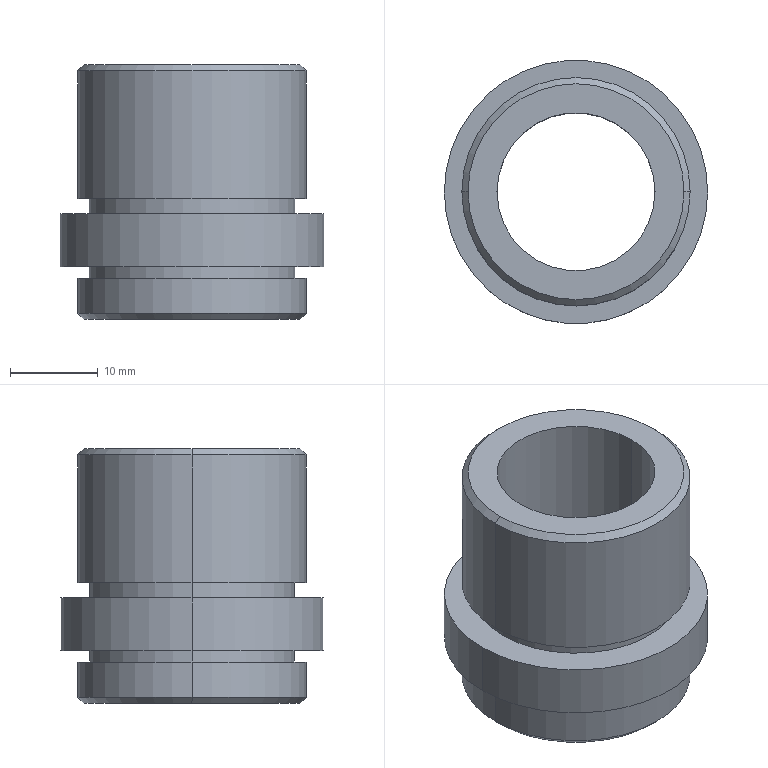Part | STEP file | TBW-1812 | 1 solid | 22 faces | box 30 x 30 x 29 mm | volume 8727 mm3 | cylinder 12 | plane 6 | cone 4 | commonest cylinder face diameters 23.4 x4 26 x4 18 x2 30 x2
STEP:
#1=CARTESIAN_POINT('',(0.,0.,0.));
#2=DIRECTION('',(0.,0.,1.));
#3=DIRECTION('',(1.,0.,0.));
#4=AXIS2_PLACEMENT_3D('',#1,#2,#3);
#5=CARTESIAN_POINT('',(-9.,0.,29.));
#6=VERTEX_POINT('',#5);
#7=CARTESIAN_POINT('',(-9.,0.,0.));
#8=VERTEX_POINT('',#7);
#9=CARTESIAN_POINT('',(-9.,0.,14.5));
#10=DIRECTION('',(0.,0.,-1.));
#11=VECTOR('',#10,1.);
#12=LINE('',#9,#11);
#13=CARTESIAN_POINT('',(0.,0.,14.5));
#14=DIRECTION('',(0.,0.,-1.));
#15=DIRECTION('',(-1.,0.,0.));
#16=AXIS2_PLACEMENT_3D('',#13,#14,#15);
#17=CYLINDRICAL_SURFACE('',#16,9.);
#18=CARTESIAN_POINT('',(6.283,0.));
#19=DIRECTION('',(0.,1.));
#20=VECTOR('',#19,1.);
#21=LINE('',#18,#20);
#22=(GEOMETRIC_REPRESENTATION_CONTEXT(2)PARAMETRIC_REPRESENTATION_CONTEXT()REPRESENTATION_CONTEXT('',''));
#23=DEFINITIONAL_REPRESENTATION('',(#21),#22);
#24=PCURVE('',#17,#23);
#25=CARTESIAN_POINT('',(0.,0.,14.5));
#26=DIRECTION('',(0.,0.,-1.));
#27=DIRECTION('',(-1.,0.,0.));
#28=AXIS2_PLACEMENT_3D('',#25,#26,#27);
#29=CYLINDRICAL_SURFACE('',#28,9.);
#30=CARTESIAN_POINT('',(0.,0.));
#31=DIRECTION('',(0.,1.));
#32=VECTOR('',#31,1.);
#33=LINE('',#30,#32);
#34=(GEOMETRIC_REPRESENTATION_CONTEXT(2)PARAMETRIC_REPRESENTATION_CONTEXT()REPRESENTATION_CONTEXT('',''));
#35=DEFINITIONAL_REPRESENTATION('',(#33),#34);
#36=PCURVE('',#29,#35);
#37=SURFACE_CURVE('',#12,(#24,#36),.PCURVE_S1.);
#38=EDGE_CURVE('',#6,#8,#37,.T.);
#39=ORIENTED_EDGE('',*,*,#38,.T.);
#40=CARTESIAN_POINT('',(9.,0.,0.));
#41=VERTEX_POINT('',#40);
#42=CARTESIAN_POINT('',(0.,0.,0.));
#43=DIRECTION('',(0.,0.,1.));
#44=DIRECTION('',(-1.,0.,0.));
#45=AXIS2_PLACEMENT_3D('',#42,#43,#44);
#46=CIRCLE('',#45,9.);
#47=CARTESIAN_POINT('',(6.283,14.5));
#48=DIRECTION('',(-1.,0.));
#49=VECTOR('',#48,1.);
#50=LINE('',#47,#49);
#51=(GEOMETRIC_REPRESENTATION_CONTEXT(2)PARAMETRIC_REPRESENTATION_CONTEXT()REPRESENTATION_CONTEXT('',''));
#52=DEFINITIONAL_REPRESENTATION('',(#50),#51);
#53=PCURVE('',#17,#52);
#54=CARTESIAN_POINT('',(0.,6.5,0.));
#55=DIRECTION('',(0.,0.,-1.));
#56=DIRECTION('',(-1.,0.,0.));
#57=AXIS2_PLACEMENT_3D('',#54,#55,#56);
#58=PLANE('',#57);
#59=CARTESIAN_POINT('',(9.,-6.5));
#60=CARTESIAN_POINT('',(9.,-22.088));
#61=CARTESIAN_POINT('',(-4.5,-14.294));
#62=CARTESIAN_POINT('',(-18.,-6.5));
#63=CARTESIAN_POINT('',(-4.5,1.294));
#64=CARTESIAN_POINT('',(9.,9.088));
#65=CARTESIAN_POINT('',(9.,-6.5));
#66=(BOUNDED_CURVE()B_SPLINE_CURVE(2,(#59,#60,#61,#62,#63,#64,#65),.UNSPECIFIED.,.T.,.F.)B_SPLINE_CURVE_WITH_KNOTS((1,2,2,2,2,1),(-2.094,0.,2.094,4.189,6.283,8.378),.UNSPECIFIED.)CURVE()GEOMETRIC_REPRESENTATION_ITEM()RATIONAL_B_SPLINE_CURVE((1.,0.5,1.,0.5,1.,0.5,1.))REPRESENTATION_ITEM(''));
#67=(GEOMETRIC_REPRESENTATION_CONTEXT(2)PARAMETRIC_REPRESENTATION_CONTEXT()REPRESENTATION_CONTEXT('',''));
#68=DEFINITIONAL_REPRESENTATION('',(#66),#67);
#69=PCURVE('',#58,#68);
#70=SURFACE_CURVE('',#46,(#53,#69),.PCURVE_S1.);
#71=EDGE_CURVE('',#8,#41,#70,.T.);
#72=ORIENTED_EDGE('',*,*,#71,.T.);
#73=CARTESIAN_POINT('',(9.,0.,29.));
#74=VERTEX_POINT('',#73);
#75=CARTESIAN_POINT('',(9.,0.,14.5));
#76=DIRECTION('',(0.,0.,-1.));
#77=VECTOR('',#76,1.);
#78=LINE('',#75,#77);
#79=CARTESIAN_POINT('',(3.142,0.));
#80=DIRECTION('',(0.,1.));
#81=VECTOR('',#80,1.);
#82=LINE('',#79,#81);
#83=(GEOMETRIC_REPRESENTATION_CONTEXT(2)PARAMETRIC_REPRESENTATION_CONTEXT()REPRESENTATION_CONTEXT('',''));
#84=DEFINITIONAL_REPRESENTATION('',(#82),#83);
#85=PCURVE('',#17,#84);
#86=CARTESIAN_POINT('',(3.142,0.));
#87=DIRECTION('',(0.,1.));
#88=VECTOR('',#87,1.);
#89=LINE('',#86,#88);
#90=(GEOMETRIC_REPRESENTATION_CONTEXT(2)PARAMETRIC_REPRESENTATION_CONTEXT()REPRESENTATION_CONTEXT('',''));
#91=DEFINITIONAL_REPRESENTATION('',(#89),#90);
#92=PCURVE('',#29,#91);
#93=SURFACE_CURVE('',#78,(#85,#92),.PCURVE_S1.);
#94=EDGE_CURVE('',#74,#41,#93,.T.);
#95=ORIENTED_EDGE('',*,*,#94,.F.);
#96=CARTESIAN_POINT('',(0.,0.,29.));
#97=DIRECTION('',(0.,0.,-1.));
#98=DIRECTION('',(-1.,0.,0.));
#99=AXIS2_PLACEMENT_3D('',#96,#97,#98);
#100=CIRCLE('',#99,9.);
#101=CARTESIAN_POINT('',(0.,-14.5));
#102=DIRECTION('',(1.,0.));
#103=VECTOR('',#102,1.);
#104=LINE('',#101,#103);
#105=(GEOMETRIC_REPRESENTATION_CONTEXT(2)PARAMETRIC_REPRESENTATION_CONTEXT()REPRESENTATION_CONTEXT('',''));
#106=DEFINITIONAL_REPRESENTATION('',(#104),#105);
#107=PCURVE('',#17,#106);
#108=CARTESIAN_POINT('',(0.,6.5,29.));
#109=DIRECTION('',(0.,0.,1.));
#110=DIRECTION('',(1.,0.,0.));
#111=AXIS2_PLACEMENT_3D('',#108,#109,#110);
#112=PLANE('',#111);
#113=CARTESIAN_POINT('',(-9.,-6.5));
#114=CARTESIAN_POINT('',(-9.,9.088));
#115=CARTESIAN_POINT('',(4.5,1.294));
#116=CARTESIAN_POINT('',(18.,-6.5));
#117=CARTESIAN_POINT('',(4.5,-14.294));
#118=CARTESIAN_POINT('',(-9.,-22.088));
#119=CARTESIAN_POINT('',(-9.,-6.5));
#120=(BOUNDED_CURVE()B_SPLINE_CURVE(2,(#113,#114,#115,#116,#117,#118,#119),.UNSPECIFIED.,.T.,.F.)B_SPLINE_CURVE_WITH_KNOTS((1,2,2,2,2,1),(-2.094,0.,2.094,4.189,6.283,8.378),.UNSPECIFIED.)CURVE()GEOMETRIC_REPRESENTATION_ITEM()RATIONAL_B_SPLINE_CURVE((1.,0.5,1.,0.5,1.,0.5,1.))REPRESENTATION_ITEM(''));
#121=(GEOMETRIC_REPRESENTATION_CONTEXT(2)PARAMETRIC_REPRESENTATION_CONTEXT()REPRESENTATION_CONTEXT('',''));
#122=DEFINITIONAL_REPRESENTATION('',(#120),#121);
#123=PCURVE('',#112,#122);
#124=SURFACE_CURVE('',#100,(#107,#123),.PCURVE_S1.);
#125=EDGE_CURVE('',#74,#6,#124,.T.);
#126=ORIENTED_EDGE('',*,*,#125,.T.);
#127=EDGE_LOOP('',(#39,#72,#95,#126));
#128=FACE_BOUND('',#127,.F.);
#129=ADVANCED_FACE('',(#128),#17,.F.);
#130=CARTESIAN_POINT('',(12.293,0.,29.));
#131=VERTEX_POINT('',#130);
#132=CARTESIAN_POINT('',(-12.293,0.,29.));
#133=VERTEX_POINT('',#132);
#134=CARTESIAN_POINT('',(0.,0.,29.));
#135=DIRECTION('',(0.,0.,1.));
#136=DIRECTION('',(-1.,0.,0.));
#137=AXIS2_PLACEMENT_3D('',#134,#135,#136);
#138=CIRCLE('',#137,12.293);
#139=CARTESIAN_POINT('',(0.,0.,28.293));
#140=DIRECTION('',(0.,0.,-1.));
#141=DIRECTION('',(-1.,0.,0.));
#142=AXIS2_PLACEMENT_3D('',#139,#140,#141);
#143=CONICAL_SURFACE('',#142,13.,0.7854);
#144=CARTESIAN_POINT('',(6.283,-0.7071));
#145=DIRECTION('',(-1.,0.));
#146=VECTOR('',#145,1.);
#147=LINE('',#144,#146);
#148=(GEOMETRIC_REPRESENTATION_CONTEXT(2)PARAMETRIC_REPRESENTATION_CONTEXT()REPRESENTATION_CONTEXT('',''));
#149=DEFINITIONAL_REPRESENTATION('',(#147),#148);
#150=PCURVE('',#143,#149);
#151=CARTESIAN_POINT('',(0.,-6.5));
#152=DIRECTION('',(-1.,0.));
#153=AXIS2_PLACEMENT_2D('',#151,#152);
#154=CIRCLE('',#153,12.293);
#155=(GEOMETRIC_REPRESENTATION_CONTEXT(2)PARAMETRIC_REPRESENTATION_CONTEXT()REPRESENTATION_CONTEXT('',''));
#156=DEFINITIONAL_REPRESENTATION('',(#154),#155);
#157=PCURVE('',#112,#156);
#158=SURFACE_CURVE('',#138,(#150,#157),.PCURVE_S1.);
#159=EDGE_CURVE('',#131,#133,#158,.T.);
#160=ORIENTED_EDGE('',*,*,#159,.F.);
#161=CARTESIAN_POINT('',(13.,0.,28.293));
#162=VERTEX_POINT('',#161);
#163=CARTESIAN_POINT('',(13.,0.,28.293));
#164=DIRECTION('',(0.7071,0.,-0.7071));
#165=VECTOR('',#164,1.);
#166=LINE('',#163,#165);
#167=CARTESIAN_POINT('',(3.142,0.));
#168=DIRECTION('',(0.,1.));
#169=VECTOR('',#168,1.);
#170=LINE('',#167,#169);
#171=(GEOMETRIC_REPRESENTATION_CONTEXT(2)PARAMETRIC_REPRESENTATION_CONTEXT()REPRESENTATION_CONTEXT('',''));
#172=DEFINITIONAL_REPRESENTATION('',(#170),#171);
#173=PCURVE('',#143,#172);
#174=CARTESIAN_POINT('',(0.,0.,28.293));
#175=DIRECTION('',(0.,0.,-1.));
#176=DIRECTION('',(-1.,0.,0.));
#177=AXIS2_PLACEMENT_3D('',#174,#175,#176);
#178=CONICAL_SURFACE('',#177,13.,0.7854);
#179=CARTESIAN_POINT('',(3.142,0.));
#180=DIRECTION('',(0.,1.));
#181=VECTOR('',#180,1.);
#182=LINE('',#179,#181);
#183=(GEOMETRIC_REPRESENTATION_CONTEXT(2)PARAMETRIC_REPRESENTATION_CONTEXT()REPRESENTATION_CONTEXT('',''));
#184=DEFINITIONAL_REPRESENTATION('',(#182),#183);
#185=PCURVE('',#178,#184);
#186=SURFACE_CURVE('',#166,(#173,#185),.PCURVE_S1.);
#187=EDGE_CURVE('',#131,#162,#186,.T.);
#188=ORIENTED_EDGE('',*,*,#187,.T.);
#189=CARTESIAN_POINT('',(-13.,0.,28.293));
#190=VERTEX_POINT('',#189);
#191=CARTESIAN_POINT('',(0.,0.,28.293));
#192=DIRECTION('',(0.,0.,1.));
#193=DIRECTION('',(0.,1.,0.));
#194=AXIS2_PLACEMENT_3D('',#191,#192,#193);
#195=CIRCLE('',#194,13.);
#196=CARTESIAN_POINT('',(7.854,0.));
#197=DIRECTION('',(-1.,0.));
#198=VECTOR('',#197,1.);
#199=LINE('',#196,#198);
#200=(GEOMETRIC_REPRESENTATION_CONTEXT(2)PARAMETRIC_REPRESENTATION_CONTEXT()REPRESENTATION_CONTEXT('',''));
#201=DEFINITIONAL_REPRESENTATION('',(#199),#200);
#202=PCURVE('',#143,#201);
#203=CARTESIAN_POINT('',(0.,0.,20.5));
#204=DIRECTION('',(0.,0.,-1.));
#205=DIRECTION('',(-1.,0.,0.));
#206=AXIS2_PLACEMENT_3D('',#203,#204,#205);
#207=CYLINDRICAL_SURFACE('',#206,13.);
#208=CARTESIAN_POINT('',(7.854,-7.793));
#209=DIRECTION('',(-1.,0.));
#210=VECTOR('',#209,1.);
#211=LINE('',#208,#210);
#212=(GEOMETRIC_REPRESENTATION_CONTEXT(2)PARAMETRIC_REPRESENTATION_CONTEXT()REPRESENTATION_CONTEXT('',''));
#213=DEFINITIONAL_REPRESENTATION('',(#211),#212);
#214=PCURVE('',#207,#213);
#215=SURFACE_CURVE('',#195,(#202,#214),.PCURVE_S1.);
#216=EDGE_CURVE('',#162,#190,#215,.T.);
#217=ORIENTED_EDGE('',*,*,#216,.T.);
#218=CARTESIAN_POINT('',(-13.,0.,28.293));
#219=DIRECTION('',(-0.7071,0.,-0.7071));
#220=VECTOR('',#219,1.);
#221=LINE('',#218,#220);
#222=CARTESIAN_POINT('',(0.,0.));
#223=DIRECTION('',(0.,1.));
#224=VECTOR('',#223,1.);
#225=LINE('',#222,#224);
#226=(GEOMETRIC_REPRESENTATION_CONTEXT(2)PARAMETRIC_REPRESENTATION_CONTEXT()REPRESENTATION_CONTEXT('',''));
#227=DEFINITIONAL_REPRESENTATION('',(#225),#226);
#228=PCURVE('',#143,#227);
#229=CARTESIAN_POINT('',(6.283,0.));
#230=DIRECTION('',(0.,1.));
#231=VECTOR('',#230,1.);
#232=LINE('',#229,#231);
#233=(GEOMETRIC_REPRESENTATION_CONTEXT(2)PARAMETRIC_REPRESENTATION_CONTEXT()REPRESENTATION_CONTEXT('',''));
#234=DEFINITIONAL_REPRESENTATION('',(#232),#233);
#235=PCURVE('',#178,#234);
#236=SURFACE_CURVE('',#221,(#228,#235),.PCURVE_S1.);
#237=EDGE_CURVE('',#133,#190,#236,.T.);
#238=ORIENTED_EDGE('',*,*,#237,.F.);
#239=EDGE_LOOP('',(#160,#188,#217,#238));
#240=FACE_BOUND('',#239,.T.);
#241=ADVANCED_FACE('',(#240),#143,.T.);
#242=CARTESIAN_POINT('',(-12.293,0.,0.));
#243=VERTEX_POINT('',#242);
#244=CARTESIAN_POINT('',(12.293,0.,0.));
#245=VERTEX_POINT('',#244);
#246=CARTESIAN_POINT('',(0.,0.,0.));
#247=DIRECTION('',(0.,0.,-1.));
#248=DIRECTION('',(1.,0.,0.));
#249=AXIS2_PLACEMENT_3D('',#246,#247,#248);
#250=CIRCLE('',#249,12.293);
#251=CARTESIAN_POINT('',(0.,0.,0.7071));
#252=DIRECTION('',(0.,0.,1.));
#253=DIRECTION('',(1.,0.,0.));
#254=AXIS2_PLACEMENT_3D('',#251,#252,#253);
#255=CONICAL_SURFACE('',#254,13.,0.7854);
#256=CARTESIAN_POINT('',(6.283,-0.7071));
#257=DIRECTION('',(-1.,0.));
#258=VECTOR('',#257,1.);
#259=LINE('',#256,#258);
#260=(GEOMETRIC_REPRESENTATION_CONTEXT(2)PARAMETRIC_REPRESENTATION_CONTEXT()REPRESENTATION_CONTEXT('',''));
#261=DEFINITIONAL_REPRESENTATION('',(#259),#260);
#262=PCURVE('',#255,#261);
#263=CARTESIAN_POINT('',(0.,-6.5));
#264=DIRECTION('',(-1.,0.));
#265=AXIS2_PLACEMENT_2D('',#263,#264);
#266=CIRCLE('',#265,12.293);
#267=(GEOMETRIC_REPRESENTATION_CONTEXT(2)PARAMETRIC_REPRESENTATION_CONTEXT()REPRESENTATION_CONTEXT('',''));
#268=DEFINITIONAL_REPRESENTATION('',(#266),#267);
#269=PCURVE('',#58,#268);
#270=SURFACE_CURVE('',#250,(#262,#269),.PCURVE_S1.);
#271=EDGE_CURVE('',#243,#245,#270,.T.);
#272=ORIENTED_EDGE('',*,*,#271,.F.);
#273=CARTESIAN_POINT('',(-13.,0.,0.7071));
#274=VERTEX_POINT('',#273);
#275=CARTESIAN_POINT('',(-13.,0.,0.7071));
#276=DIRECTION('',(-0.7071,0.,0.7071));
#277=VECTOR('',#276,1.);
#278=LINE('',#275,#277);
#279=CARTESIAN_POINT('',(3.142,0.));
#280=DIRECTION('',(0.,1.));
#281=VECTOR('',#280,1.);
#282=LINE('',#279,#281);
#283=(GEOMETRIC_REPRESENTATION_CONTEXT(2)PARAMETRIC_REPRESENTATION_CONTEXT()REPRESENTATION_CONTEXT('',''));
#284=DEFINITIONAL_REPRESENTATION('',(#282),#283);
#285=PCURVE('',#255,#284);
#286=CARTESIAN_POINT('',(0.,0.,0.7071));
#287=DIRECTION('',(0.,0.,1.));
#288=DIRECTION('',(1.,0.,0.));
#289=AXIS2_PLACEMENT_3D('',#286,#287,#288);
#290=CONICAL_SURFACE('',#289,13.,0.7854);
#291=CARTESIAN_POINT('',(3.142,0.));
#292=DIRECTION('',(0.,1.));
#293=VECTOR('',#292,1.);
#294=LINE('',#291,#293);
#295=(GEOMETRIC_REPRESENTATION_CONTEXT(2)PARAMETRIC_REPRESENTATION_CONTEXT()REPRESENTATION_CONTEXT('',''));
#296=DEFINITIONAL_REPRESENTATION('',(#294),#295);
#297=PCURVE('',#290,#296);
#298=SURFACE_CURVE('',#278,(#285,#297),.PCURVE_S1.);
#299=EDGE_CURVE('',#243,#274,#298,.T.);
#300=ORIENTED_EDGE('',*,*,#299,.T.);
#301=CARTESIAN_POINT('',(13.,0.,0.7071));
#302=VERTEX_POINT('',#301);
#303=CARTESIAN_POINT('',(0.,0.,0.7071));
#304=DIRECTION('',(0.,0.,-1.));
#305=DIRECTION('',(0.,1.,0.));
#306=AXIS2_PLACEMENT_3D('',#303,#304,#305);
#307=CIRCLE('',#306,13.);
#308=CARTESIAN_POINT('',(7.854,0.));
#309=DIRECTION('',(-1.,0.));
#310=VECTOR('',#309,1.);
#311=LINE('',#308,#310);
#312=(GEOMETRIC_REPRESENTATION_CONTEXT(2)PARAMETRIC_REPRESENTATION_CONTEXT()REPRESENTATION_CONTEXT('',''));
#313=DEFINITIONAL_REPRESENTATION('',(#311),#312);
#314=PCURVE('',#255,#313);
#315=CARTESIAN_POINT('',(0.,0.,3.));
#316=DIRECTION('',(0.,0.,-1.));
#317=DIRECTION('',(-1.,0.,0.));
#318=AXIS2_PLACEMENT_3D('',#315,#316,#317);
#319=CYLINDRICAL_SURFACE('',#318,13.);
#320=CARTESIAN_POINT('',(-4.712,2.293));
#321=DIRECTION('',(1.,0.));
#322=VECTOR('',#321,1.);
#323=LINE('',#320,#322);
#324=(GEOMETRIC_REPRESENTATION_CONTEXT(2)PARAMETRIC_REPRESENTATION_CONTEXT()REPRESENTATION_CONTEXT('',''));
#325=DEFINITIONAL_REPRESENTATION('',(#323),#324);
#326=PCURVE('',#319,#325);
#327=SURFACE_CURVE('',#307,(#314,#326),.PCURVE_S1.);
#328=EDGE_CURVE('',#274,#302,#327,.T.);
#329=ORIENTED_EDGE('',*,*,#328,.T.);
#330=CARTESIAN_POINT('',(13.,0.,0.7071));
#331=DIRECTION('',(0.7071,0.,0.7071));
#332=VECTOR('',#331,1.);
#333=LINE('',#330,#332);
#334=CARTESIAN_POINT('',(0.,0.));
#335=DIRECTION('',(0.,1.));
#336=VECTOR('',#335,1.);
#337=LINE('',#334,#336);
#338=(GEOMETRIC_REPRESENTATION_CONTEXT(2)PARAMETRIC_REPRESENTATION_CONTEXT()REPRESENTATION_CONTEXT('',''));
#339=DEFINITIONAL_REPRESENTATION('',(#337),#338);
#340=PCURVE('',#255,#339);
#341=CARTESIAN_POINT('',(6.283,0.));
#342=DIRECTION('',(0.,1.));
#343=VECTOR('',#342,1.);
#344=LINE('',#341,#343);
#345=(GEOMETRIC_REPRESENTATION_CONTEXT(2)PARAMETRIC_REPRESENTATION_CONTEXT()REPRESENTATION_CONTEXT('',''));
#346=DEFINITIONAL_REPRESENTATION('',(#344),#345);
#347=PCURVE('',#290,#346);
#348=SURFACE_CURVE('',#333,(#340,#347),.PCURVE_S1.);
#349=EDGE_CURVE('',#245,#302,#348,.T.);
#350=ORIENTED_EDGE('',*,*,#349,.F.);
#351=EDGE_LOOP('',(#272,#300,#329,#350));
#352=FACE_BOUND('',#351,.T.);
#353=ADVANCED_FACE('',(#352),#255,.T.);
#354=ORIENTED_EDGE('',*,*,#216,.F.);
#355=CARTESIAN_POINT('',(13.,0.,13.733));
#356=VERTEX_POINT('',#355);
#357=CARTESIAN_POINT('',(13.,0.,20.5));
#358=DIRECTION('',(0.,0.,-1.));
#359=VECTOR('',#358,1.);
#360=LINE('',#357,#359);
#361=CARTESIAN_POINT('',(3.142,0.));
#362=DIRECTION('',(0.,1.));
#363=VECTOR('',#362,1.);
#364=LINE('',#361,#363);
#365=(GEOMETRIC_REPRESENTATION_CONTEXT(2)PARAMETRIC_REPRESENTATION_CONTEXT()REPRESENTATION_CONTEXT('',''));
#366=DEFINITIONAL_REPRESENTATION('',(#364),#365);
#367=PCURVE('',#207,#366);
#368=CARTESIAN_POINT('',(0.,0.,20.5));
#369=DIRECTION('',(0.,0.,-1.));
#370=DIRECTION('',(-1.,0.,0.));
#371=AXIS2_PLACEMENT_3D('',#368,#369,#370);
#372=CYLINDRICAL_SURFACE('',#371,13.);
#373=CARTESIAN_POINT('',(3.142,0.));
#374=DIRECTION('',(0.,1.));
#375=VECTOR('',#374,1.);
#376=LINE('',#373,#375);
#377=(GEOMETRIC_REPRESENTATION_CONTEXT(2)PARAMETRIC_REPRESENTATION_CONTEXT()REPRESENTATION_CONTEXT('',''));
#378=DEFINITIONAL_REPRESENTATION('',(#376),#377);
#379=PCURVE('',#372,#378);
#380=SURFACE_CURVE('',#360,(#367,#379),.PCURVE_S1.);
#381=EDGE_CURVE('',#162,#356,#380,.T.);
#382=ORIENTED_EDGE('',*,*,#381,.T.);
#383=CARTESIAN_POINT('',(-13.,0.,13.733));
#384=VERTEX_POINT('',#383);
#385=CARTESIAN_POINT('',(0.,0.,13.733));
#386=DIRECTION('',(0.,0.,1.));
#387=DIRECTION('',(-1.,0.,0.));
#388=AXIS2_PLACEMENT_3D('',#385,#386,#387);
#389=CIRCLE('',#388,13.);
#390=CARTESIAN_POINT('',(6.283,6.767));
#391=DIRECTION('',(-1.,0.));
#392=VECTOR('',#391,1.);
#393=LINE('',#390,#392);
#394=(GEOMETRIC_REPRESENTATION_CONTEXT(2)PARAMETRIC_REPRESENTATION_CONTEXT()REPRESENTATION_CONTEXT('',''));
#395=DEFINITIONAL_REPRESENTATION('',(#393),#394);
#396=PCURVE('',#207,#395);
#397=CARTESIAN_POINT('',(0.,12.35,13.733));
#398=DIRECTION('',(0.,0.,1.));
#399=DIRECTION('',(1.,0.,0.));
#400=AXIS2_PLACEMENT_3D('',#397,#398,#399);
#401=PLANE('',#400);
#402=CARTESIAN_POINT('',(0.,-12.35));
#403=DIRECTION('',(-1.,0.));
#404=AXIS2_PLACEMENT_2D('',#402,#403);
#405=CIRCLE('',#404,13.);
#406=(GEOMETRIC_REPRESENTATION_CONTEXT(2)PARAMETRIC_REPRESENTATION_CONTEXT()REPRESENTATION_CONTEXT('',''));
#407=DEFINITIONAL_REPRESENTATION('',(#405),#406);
#408=PCURVE('',#401,#407);
#409=SURFACE_CURVE('',#389,(#396,#408),.PCURVE_S1.);
#410=EDGE_CURVE('',#356,#384,#409,.T.);
#411=ORIENTED_EDGE('',*,*,#410,.T.);
#412=CARTESIAN_POINT('',(-13.,0.,20.5));
#413=DIRECTION('',(0.,0.,-1.));
#414=VECTOR('',#413,1.);
#415=LINE('',#412,#414);
#416=CARTESIAN_POINT('',(0.,0.));
#417=DIRECTION('',(0.,1.));
#418=VECTOR('',#417,1.);
#419=LINE('',#416,#418);
#420=(GEOMETRIC_REPRESENTATION_CONTEXT(2)PARAMETRIC_REPRESENTATION_CONTEXT()REPRESENTATION_CONTEXT('',''));
#421=DEFINITIONAL_REPRESENTATION('',(#419),#420);
#422=PCURVE('',#207,#421);
#423=CARTESIAN_POINT('',(6.283,0.));
#424=DIRECTION('',(0.,1.));
#425=VECTOR('',#424,1.);
#426=LINE('',#423,#425);
#427=(GEOMETRIC_REPRESENTATION_CONTEXT(2)PARAMETRIC_REPRESENTATION_CONTEXT()REPRESENTATION_CONTEXT('',''));
#428=DEFINITIONAL_REPRESENTATION('',(#426),#427);
#429=PCURVE('',#372,#428);
#430=SURFACE_CURVE('',#415,(#422,#429),.PCURVE_S1.);
#431=EDGE_CURVE('',#190,#384,#430,.T.);
#432=ORIENTED_EDGE('',*,*,#431,.F.);
#433=EDGE_LOOP('',(#354,#382,#411,#432));
#434=FACE_BOUND('',#433,.T.);
#435=ADVANCED_FACE('',(#434),#207,.T.);
#436=CARTESIAN_POINT('',(-13.,0.,4.7));
#437=VERTEX_POINT('',#436);
#438=CARTESIAN_POINT('',(13.,0.,4.7));
#439=VERTEX_POINT('',#438);
#440=CARTESIAN_POINT('',(0.,0.,4.7));
#441=DIRECTION('',(0.,0.,-1.));
#442=DIRECTION('',(-1.,0.,0.));
#443=AXIS2_PLACEMENT_3D('',#440,#441,#442);
#444=CIRCLE('',#443,13.);
#445=CARTESIAN_POINT('',(0.,-1.7));
#446=DIRECTION('',(1.,0.));
#447=VECTOR('',#446,1.);
#448=LINE('',#445,#447);
#449=(GEOMETRIC_REPRESENTATION_CONTEXT(2)PARAMETRIC_REPRESENTATION_CONTEXT()REPRESENTATION_CONTEXT('',''));
#450=DEFINITIONAL_REPRESENTATION('',(#448),#449);
#451=PCURVE('',#319,#450);
#452=CARTESIAN_POINT('',(0.,12.35,4.7));
#453=DIRECTION('',(0.,0.,-1.));
#454=DIRECTION('',(-1.,0.,0.));
#455=AXIS2_PLACEMENT_3D('',#452,#453,#454);
#456=PLANE('',#455);
#457=CARTESIAN_POINT('',(0.,-12.35));
#458=DIRECTION('',(1.,0.));
#459=AXIS2_PLACEMENT_2D('',#457,#458);
#460=CIRCLE('',#459,13.);
#461=(GEOMETRIC_REPRESENTATION_CONTEXT(2)PARAMETRIC_REPRESENTATION_CONTEXT()REPRESENTATION_CONTEXT('',''));
#462=DEFINITIONAL_REPRESENTATION('',(#460),#461);
#463=PCURVE('',#456,#462);
#464=SURFACE_CURVE('',#444,(#451,#463),.PCURVE_S1.);
#465=EDGE_CURVE('',#437,#439,#464,.T.);
#466=ORIENTED_EDGE('',*,*,#465,.T.);
#467=CARTESIAN_POINT('',(13.,0.,3.));
#468=DIRECTION('',(0.,0.,-1.));
#469=VECTOR('',#468,1.);
#470=LINE('',#467,#469);
#471=CARTESIAN_POINT('',(3.142,0.));
#472=DIRECTION('',(0.,1.));
#473=VECTOR('',#472,1.);
#474=LINE('',#471,#473);
#475=(GEOMETRIC_REPRESENTATION_CONTEXT(2)PARAMETRIC_REPRESENTATION_CONTEXT()REPRESENTATION_CONTEXT('',''));
#476=DEFINITIONAL_REPRESENTATION('',(#474),#475);
#477=PCURVE('',#319,#476);
#478=CARTESIAN_POINT('',(0.,0.,3.));
#479=DIRECTION('',(0.,0.,-1.));
#480=DIRECTION('',(-1.,0.,0.));
#481=AXIS2_PLACEMENT_3D('',#478,#479,#480);
#482=CYLINDRICAL_SURFACE('',#481,13.);
#483=CARTESIAN_POINT('',(3.142,0.));
#484=DIRECTION('',(0.,1.));
#485=VECTOR('',#484,1.);
#486=LINE('',#483,#485);
#487=(GEOMETRIC_REPRESENTATION_CONTEXT(2)PARAMETRIC_REPRESENTATION_CONTEXT()REPRESENTATION_CONTEXT('',''));
#488=DEFINITIONAL_REPRESENTATION('',(#486),#487);
#489=PCURVE('',#482,#488);
#490=SURFACE_CURVE('',#470,(#477,#489),.PCURVE_S1.);
#491=EDGE_CURVE('',#439,#302,#490,.T.);
#492=ORIENTED_EDGE('',*,*,#491,.T.);
#493=ORIENTED_EDGE('',*,*,#328,.F.);
#494=CARTESIAN_POINT('',(-13.,0.,3.));
#495=DIRECTION('',(0.,0.,-1.));
#496=VECTOR('',#495,1.);
#497=LINE('',#494,#496);
#498=CARTESIAN_POINT('',(0.,0.));
#499=DIRECTION('',(0.,1.));
#500=VECTOR('',#499,1.);
#501=LINE('',#498,#500);
#502=(GEOMETRIC_REPRESENTATION_CONTEXT(2)PARAMETRIC_REPRESENTATION_CONTEXT()REPRESENTATION_CONTEXT('',''));
#503=DEFINITIONAL_REPRESENTATION('',(#501),#502);
#504=PCURVE('',#319,#503);
#505=CARTESIAN_POINT('',(6.283,0.));
#506=DIRECTION('',(0.,1.));
#507=VECTOR('',#506,1.);
#508=LINE('',#505,#507);
#509=(GEOMETRIC_REPRESENTATION_CONTEXT(2)PARAMETRIC_REPRESENTATION_CONTEXT()REPRESENTATION_CONTEXT('',''));
#510=DEFINITIONAL_REPRESENTATION('',(#508),#509);
#511=PCURVE('',#482,#510);
#512=SURFACE_CURVE('',#497,(#504,#511),.PCURVE_S1.);
#513=EDGE_CURVE('',#437,#274,#512,.T.);
#514=ORIENTED_EDGE('',*,*,#513,.F.);
#515=EDGE_LOOP('',(#466,#492,#493,#514));
#516=FACE_BOUND('',#515,.T.);
#517=ADVANCED_FACE('',(#516),#319,.T.);
#518=CARTESIAN_POINT('',(-11.7,0.,13.733));
#519=VERTEX_POINT('',#518);
#520=CARTESIAN_POINT('',(11.7,0.,13.733));
#521=VERTEX_POINT('',#520);
#522=CARTESIAN_POINT('',(0.,0.,13.733));
#523=DIRECTION('',(0.,0.,-1.));
#524=DIRECTION('',(-1.,0.,0.));
#525=AXIS2_PLACEMENT_3D('',#522,#523,#524);
#526=CIRCLE('',#525,11.7);
#527=CARTESIAN_POINT('',(0.,0.,12.867));
#528=DIRECTION('',(0.,0.,-1.));
#529=DIRECTION('',(-1.,0.,0.));
#530=AXIS2_PLACEMENT_3D('',#527,#528,#529);
#531=CYLINDRICAL_SURFACE('',#530,11.7);
#532=CARTESIAN_POINT('',(0.,-0.8667));
#533=DIRECTION('',(1.,0.));
#534=VECTOR('',#533,1.);
#535=LINE('',#532,#534);
#536=(GEOMETRIC_REPRESENTATION_CONTEXT(2)PARAMETRIC_REPRESENTATION_CONTEXT()REPRESENTATION_CONTEXT('',''));
#537=DEFINITIONAL_REPRESENTATION('',(#535),#536);
#538=PCURVE('',#531,#537);
#539=CARTESIAN_POINT('',(-11.7,-12.35));
#540=CARTESIAN_POINT('',(-11.7,7.915));
#541=CARTESIAN_POINT('',(5.85,-2.218));
#542=CARTESIAN_POINT('',(23.4,-12.35));
#543=CARTESIAN_POINT('',(5.85,-22.482));
#544=CARTESIAN_POINT('',(-11.7,-32.615));
#545=CARTESIAN_POINT('',(-11.7,-12.35));
#546=(BOUNDED_CURVE()B_SPLINE_CURVE(2,(#539,#540,#541,#542,#543,#544,#545),.UNSPECIFIED.,.T.,.F.)B_SPLINE_CURVE_WITH_KNOTS((1,2,2,2,2,1),(-2.094,0.,2.094,4.189,6.283,8.378),.UNSPECIFIED.)CURVE()GEOMETRIC_REPRESENTATION_ITEM()RATIONAL_B_SPLINE_CURVE((1.,0.5,1.,0.5,1.,0.5,1.))REPRESENTATION_ITEM(''));
#547=(GEOMETRIC_REPRESENTATION_CONTEXT(2)PARAMETRIC_REPRESENTATION_CONTEXT()REPRESENTATION_CONTEXT('',''));
#548=DEFINITIONAL_REPRESENTATION('',(#546),#547);
#549=PCURVE('',#401,#548);
#550=SURFACE_CURVE('',#526,(#538,#549),.PCURVE_S1.);
#551=EDGE_CURVE('',#519,#521,#550,.T.);
#552=ORIENTED_EDGE('',*,*,#551,.T.);
#553=CARTESIAN_POINT('',(11.7,0.,12.));
#554=VERTEX_POINT('',#553);
#555=CARTESIAN_POINT('',(11.7,0.,12.867));
#556=DIRECTION('',(0.,0.,-1.));
#557=VECTOR('',#556,1.);
#558=LINE('',#555,#557);
#559=CARTESIAN_POINT('',(3.142,0.));
#560=DIRECTION('',(0.,1.));
#561=VECTOR('',#560,1.);
#562=LINE('',#559,#561);
#563=(GEOMETRIC_REPRESENTATION_CONTEXT(2)PARAMETRIC_REPRESENTATION_CONTEXT()REPRESENTATION_CONTEXT('',''));
#564=DEFINITIONAL_REPRESENTATION('',(#562),#563);
#565=PCURVE('',#531,#564);
#566=CARTESIAN_POINT('',(0.,0.,12.867));
#567=DIRECTION('',(0.,0.,-1.));
#568=DIRECTION('',(-1.,0.,0.));
#569=AXIS2_PLACEMENT_3D('',#566,#567,#568);
#570=CYLINDRICAL_SURFACE('',#569,11.7);
#571=CARTESIAN_POINT('',(3.142,0.));
#572=DIRECTION('',(0.,1.));
#573=VECTOR('',#572,1.);
#574=LINE('',#571,#573);
#575=(GEOMETRIC_REPRESENTATION_CONTEXT(2)PARAMETRIC_REPRESENTATION_CONTEXT()REPRESENTATION_CONTEXT('',''));
#576=DEFINITIONAL_REPRESENTATION('',(#574),#575);
#577=PCURVE('',#570,#576);
#578=SURFACE_CURVE('',#558,(#565,#577),.PCURVE_S1.);
#579=EDGE_CURVE('',#521,#554,#578,.T.);
#580=ORIENTED_EDGE('',*,*,#579,.T.);
#581=CARTESIAN_POINT('',(-11.7,0.,12.));
#582=VERTEX_POINT('',#581);
#583=CARTESIAN_POINT('',(0.,0.,12.));
#584=DIRECTION('',(0.,0.,1.));
#585=DIRECTION('',(-1.,0.,0.));
#586=AXIS2_PLACEMENT_3D('',#583,#584,#585);
#587=CIRCLE('',#586,11.7);
#588=CARTESIAN_POINT('',(6.283,0.8667));
#589=DIRECTION('',(-1.,0.));
#590=VECTOR('',#589,1.);
#591=LINE('',#588,#590);
#592=(GEOMETRIC_REPRESENTATION_CONTEXT(2)PARAMETRIC_REPRESENTATION_CONTEXT()REPRESENTATION_CONTEXT('',''));
#593=DEFINITIONAL_REPRESENTATION('',(#591),#592);
#594=PCURVE('',#531,#593);
#595=CARTESIAN_POINT('',(0.,7.5,12.));
#596=DIRECTION('',(0.,0.,1.));
#597=DIRECTION('',(1.,0.,0.));
#598=AXIS2_PLACEMENT_3D('',#595,#596,#597);
#599=PLANE('',#598);
#600=CARTESIAN_POINT('',(0.,-7.5));
#601=DIRECTION('',(-1.,0.));
#602=AXIS2_PLACEMENT_2D('',#600,#601);
#603=CIRCLE('',#602,11.7);
#604=(GEOMETRIC_REPRESENTATION_CONTEXT(2)PARAMETRIC_REPRESENTATION_CONTEXT()REPRESENTATION_CONTEXT('',''));
#605=DEFINITIONAL_REPRESENTATION('',(#603),#604);
#606=PCURVE('',#599,#605);
#607=SURFACE_CURVE('',#587,(#594,#606),.PCURVE_S1.);
#608=EDGE_CURVE('',#554,#582,#607,.T.);
#609=ORIENTED_EDGE('',*,*,#608,.T.);
#610=CARTESIAN_POINT('',(-11.7,0.,12.867));
#611=DIRECTION('',(0.,0.,-1.));
#612=VECTOR('',#611,1.);
#613=LINE('',#610,#612);
#614=CARTESIAN_POINT('',(0.,0.));
#615=DIRECTION('',(0.,1.));
#616=VECTOR('',#615,1.);
#617=LINE('',#614,#616);
#618=(GEOMETRIC_REPRESENTATION_CONTEXT(2)PARAMETRIC_REPRESENTATION_CONTEXT()REPRESENTATION_CONTEXT('',''));
#619=DEFINITIONAL_REPRESENTATION('',(#617),#618);
#620=PCURVE('',#531,#619);
#621=CARTESIAN_POINT('',(6.283,0.));
#622=DIRECTION('',(0.,1.));
#623=VECTOR('',#622,1.);
#624=LINE('',#621,#623);
#625=(GEOMETRIC_REPRESENTATION_CONTEXT(2)PARAMETRIC_REPRESENTATION_CONTEXT()REPRESENTATION_CONTEXT('',''));
#626=DEFINITIONAL_REPRESENTATION('',(#624),#625);
#627=PCURVE('',#570,#626);
#628=SURFACE_CURVE('',#613,(#620,#627),.PCURVE_S1.);
#629=EDGE_CURVE('',#519,#582,#628,.T.);
#630=ORIENTED_EDGE('',*,*,#629,.F.);
#631=EDGE_LOOP('',(#552,#580,#609,#630));
#632=FACE_BOUND('',#631,.T.);
#633=ADVANCED_FACE('',(#632),#531,.T.);
#634=CARTESIAN_POINT('',(-11.7,0.,6.));
#635=VERTEX_POINT('',#634);
#636=CARTESIAN_POINT('',(11.7,0.,6.));
#637=VERTEX_POINT('',#636);
#638=CARTESIAN_POINT('',(0.,0.,6.));
#639=DIRECTION('',(0.,0.,-1.));
#640=DIRECTION('',(-1.,0.,0.));
#641=AXIS2_PLACEMENT_3D('',#638,#639,#640);
#642=CIRCLE('',#641,11.7);
#643=CARTESIAN_POINT('',(0.,0.,5.35));
#644=DIRECTION('',(0.,0.,-1.));
#645=DIRECTION('',(-1.,0.,0.));
#646=AXIS2_PLACEMENT_3D('',#643,#644,#645);
#647=CYLINDRICAL_SURFACE('',#646,11.7);
#648=CARTESIAN_POINT('',(0.,-0.65));
#649=DIRECTION('',(1.,0.));
#650=VECTOR('',#649,1.);
#651=LINE('',#648,#650);
#652=(GEOMETRIC_REPRESENTATION_CONTEXT(2)PARAMETRIC_REPRESENTATION_CONTEXT()REPRESENTATION_CONTEXT('',''));
#653=DEFINITIONAL_REPRESENTATION('',(#651),#652);
#654=PCURVE('',#647,#653);
#655=CARTESIAN_POINT('',(0.,7.5,6.));
#656=DIRECTION('',(0.,0.,-1.));
#657=DIRECTION('',(-1.,0.,0.));
#658=AXIS2_PLACEMENT_3D('',#655,#656,#657);
#659=PLANE('',#658);
#660=CARTESIAN_POINT('',(0.,-7.5));
#661=DIRECTION('',(1.,0.));
#662=AXIS2_PLACEMENT_2D('',#660,#661);
#663=CIRCLE('',#662,11.7);
#664=(GEOMETRIC_REPRESENTATION_CONTEXT(2)PARAMETRIC_REPRESENTATION_CONTEXT()REPRESENTATION_CONTEXT('',''));
#665=DEFINITIONAL_REPRESENTATION('',(#663),#664);
#666=PCURVE('',#659,#665);
#667=SURFACE_CURVE('',#642,(#654,#666),.PCURVE_S1.);
#668=EDGE_CURVE('',#635,#637,#667,.T.);
#669=ORIENTED_EDGE('',*,*,#668,.T.);
#670=CARTESIAN_POINT('',(11.7,0.,4.7));
#671=VERTEX_POINT('',#670);
#672=CARTESIAN_POINT('',(11.7,0.,5.35));
#673=DIRECTION('',(0.,0.,-1.));
#674=VECTOR('',#673,1.);
#675=LINE('',#672,#674);
#676=CARTESIAN_POINT('',(3.142,0.));
#677=DIRECTION('',(0.,1.));
#678=VECTOR('',#677,1.);
#679=LINE('',#676,#678);
#680=(GEOMETRIC_REPRESENTATION_CONTEXT(2)PARAMETRIC_REPRESENTATION_CONTEXT()REPRESENTATION_CONTEXT('',''));
#681=DEFINITIONAL_REPRESENTATION('',(#679),#680);
#682=PCURVE('',#647,#681);
#683=CARTESIAN_POINT('',(0.,0.,5.35));
#684=DIRECTION('',(0.,0.,-1.));
#685=DIRECTION('',(-1.,0.,0.));
#686=AXIS2_PLACEMENT_3D('',#683,#684,#685);
#687=CYLINDRICAL_SURFACE('',#686,11.7);
#688=CARTESIAN_POINT('',(3.142,0.));
#689=DIRECTION('',(0.,1.));
#690=VECTOR('',#689,1.);
#691=LINE('',#688,#690);
#692=(GEOMETRIC_REPRESENTATION_CONTEXT(2)PARAMETRIC_REPRESENTATION_CONTEXT()REPRESENTATION_CONTEXT('',''));
#693=DEFINITIONAL_REPRESENTATION('',(#691),#692);
#694=PCURVE('',#687,#693);
#695=SURFACE_CURVE('',#675,(#682,#694),.PCURVE_S1.);
#696=EDGE_CURVE('',#637,#671,#695,.T.);
#697=ORIENTED_EDGE('',*,*,#696,.T.);
#698=CARTESIAN_POINT('',(-11.7,0.,4.7));
#699=VERTEX_POINT('',#698);
#700=CARTESIAN_POINT('',(0.,0.,4.7));
#701=DIRECTION('',(0.,0.,1.));
#702=DIRECTION('',(-1.,0.,0.));
#703=AXIS2_PLACEMENT_3D('',#700,#701,#702);
#704=CIRCLE('',#703,11.7);
#705=CARTESIAN_POINT('',(6.283,0.65));
#706=DIRECTION('',(-1.,0.));
#707=VECTOR('',#706,1.);
#708=LINE('',#705,#707);
#709=(GEOMETRIC_REPRESENTATION_CONTEXT(2)PARAMETRIC_REPRESENTATION_CONTEXT()REPRESENTATION_CONTEXT('',''));
#710=DEFINITIONAL_REPRESENTATION('',(#708),#709);
#711=PCURVE('',#647,#710);
#712=CARTESIAN_POINT('',(11.7,-12.35));
#713=CARTESIAN_POINT('',(11.7,-32.615));
#714=CARTESIAN_POINT('',(-5.85,-22.482));
#715=CARTESIAN_POINT('',(-23.4,-12.35));
#716=CARTESIAN_POINT('',(-5.85,-2.218));
#717=CARTESIAN_POINT('',(11.7,7.915));
#718=CARTESIAN_POINT('',(11.7,-12.35));
#719=(BOUNDED_CURVE()B_SPLINE_CURVE(2,(#712,#713,#714,#715,#716,#717,#718),.UNSPECIFIED.,.T.,.F.)B_SPLINE_CURVE_WITH_KNOTS((1,2,2,2,2,1),(-2.094,0.,2.094,4.189,6.283,8.378),.UNSPECIFIED.)CURVE()GEOMETRIC_REPRESENTATION_ITEM()RATIONAL_B_SPLINE_CURVE((1.,0.5,1.,0.5,1.,0.5,1.))REPRESENTATION_ITEM(''));
#720=(GEOMETRIC_REPRESENTATION_CONTEXT(2)PARAMETRIC_REPRESENTATION_CONTEXT()REPRESENTATION_CONTEXT('',''));
#721=DEFINITIONAL_REPRESENTATION('',(#719),#720);
#722=PCURVE('',#456,#721);
#723=SURFACE_CURVE('',#704,(#711,#722),.PCURVE_S1.);
#724=EDGE_CURVE('',#671,#699,#723,.T.);
#725=ORIENTED_EDGE('',*,*,#724,.T.);
#726=CARTESIAN_POINT('',(-11.7,0.,5.35));
#727=DIRECTION('',(0.,0.,-1.));
#728=VECTOR('',#727,1.);
#729=LINE('',#726,#728);
#730=CARTESIAN_POINT('',(0.,0.));
#731=DIRECTION('',(0.,1.));
#732=VECTOR('',#731,1.);
#733=LINE('',#730,#732);
#734=(GEOMETRIC_REPRESENTATION_CONTEXT(2)PARAMETRIC_REPRESENTATION_CONTEXT()REPRESENTATION_CONTEXT('',''));
#735=DEFINITIONAL_REPRESENTATION('',(#733),#734);
#736=PCURVE('',#647,#735);
#737=CARTESIAN_POINT('',(6.283,0.));
#738=DIRECTION('',(0.,1.));
#739=VECTOR('',#738,1.);
#740=LINE('',#737,#739);
#741=(GEOMETRIC_REPRESENTATION_CONTEXT(2)PARAMETRIC_REPRESENTATION_CONTEXT()REPRESENTATION_CONTEXT('',''));
#742=DEFINITIONAL_REPRESENTATION('',(#740),#741);
#743=PCURVE('',#687,#742);
#744=SURFACE_CURVE('',#729,(#736,#743),.PCURVE_S1.);
#745=EDGE_CURVE('',#635,#699,#744,.T.);
#746=ORIENTED_EDGE('',*,*,#745,.F.);
#747=EDGE_LOOP('',(#669,#697,#725,#746));
#748=FACE_BOUND('',#747,.T.);
#749=ADVANCED_FACE('',(#748),#647,.T.);
#750=CARTESIAN_POINT('',(15.,0.,12.));
#751=VERTEX_POINT('',#750);
#752=CARTESIAN_POINT('',(-15.,0.,12.));
#753=VERTEX_POINT('',#752);
#754=CARTESIAN_POINT('',(0.,0.,12.));
#755=DIRECTION('',(0.,0.,1.));
#756=DIRECTION('',(-1.,0.,0.));
#757=AXIS2_PLACEMENT_3D('',#754,#755,#756);
#758=CIRCLE('',#757,15.);
#759=CARTESIAN_POINT('',(0.,0.,9.));
#760=DIRECTION('',(0.,0.,-1.));
#761=DIRECTION('',(-1.,0.,0.));
#762=AXIS2_PLACEMENT_3D('',#759,#760,#761);
#763=CYLINDRICAL_SURFACE('',#762,15.);
#764=CARTESIAN_POINT('',(6.283,-3.));
#765=DIRECTION('',(-1.,0.));
#766=VECTOR('',#765,1.);
#767=LINE('',#764,#766);
#768=(GEOMETRIC_REPRESENTATION_CONTEXT(2)PARAMETRIC_REPRESENTATION_CONTEXT()REPRESENTATION_CONTEXT('',''));
#769=DEFINITIONAL_REPRESENTATION('',(#767),#768);
#770=PCURVE('',#763,#769);
#771=CARTESIAN_POINT('',(0.,-7.5));
#772=DIRECTION('',(-1.,0.));
#773=AXIS2_PLACEMENT_2D('',#771,#772);
#774=CIRCLE('',#773,15.);
#775=(GEOMETRIC_REPRESENTATION_CONTEXT(2)PARAMETRIC_REPRESENTATION_CONTEXT()REPRESENTATION_CONTEXT('',''));
#776=DEFINITIONAL_REPRESENTATION('',(#774),#775);
#777=PCURVE('',#599,#776);
#778=SURFACE_CURVE('',#758,(#770,#777),.PCURVE_S1.);
#779=EDGE_CURVE('',#751,#753,#778,.T.);
#780=ORIENTED_EDGE('',*,*,#779,.F.);
#781=CARTESIAN_POINT('',(15.,0.,6.));
#782=VERTEX_POINT('',#781);
#783=CARTESIAN_POINT('',(15.,0.,9.));
#784=DIRECTION('',(0.,0.,-1.));
#785=VECTOR('',#784,1.);
#786=LINE('',#783,#785);
#787=CARTESIAN_POINT('',(3.142,0.));
#788=DIRECTION('',(0.,1.));
#789=VECTOR('',#788,1.);
#790=LINE('',#787,#789);
#791=(GEOMETRIC_REPRESENTATION_CONTEXT(2)PARAMETRIC_REPRESENTATION_CONTEXT()REPRESENTATION_CONTEXT('',''));
#792=DEFINITIONAL_REPRESENTATION('',(#790),#791);
#793=PCURVE('',#763,#792);
#794=CARTESIAN_POINT('',(0.,0.,9.));
#795=DIRECTION('',(0.,0.,-1.));
#796=DIRECTION('',(-1.,0.,0.));
#797=AXIS2_PLACEMENT_3D('',#794,#795,#796);
#798=CYLINDRICAL_SURFACE('',#797,15.);
#799=CARTESIAN_POINT('',(3.142,0.));
#800=DIRECTION('',(0.,1.));
#801=VECTOR('',#800,1.);
#802=LINE('',#799,#801);
#803=(GEOMETRIC_REPRESENTATION_CONTEXT(2)PARAMETRIC_REPRESENTATION_CONTEXT()REPRESENTATION_CONTEXT('',''));
#804=DEFINITIONAL_REPRESENTATION('',(#802),#803);
#805=PCURVE('',#798,#804);
#806=SURFACE_CURVE('',#786,(#793,#805),.PCURVE_S1.);
#807=EDGE_CURVE('',#751,#782,#806,.T.);
#808=ORIENTED_EDGE('',*,*,#807,.T.);
#809=CARTESIAN_POINT('',(-15.,0.,6.));
#810=VERTEX_POINT('',#809);
#811=CARTESIAN_POINT('',(0.,0.,6.));
#812=DIRECTION('',(0.,0.,-1.));
#813=DIRECTION('',(-1.,0.,0.));
#814=AXIS2_PLACEMENT_3D('',#811,#812,#813);
#815=CIRCLE('',#814,15.);
#816=CARTESIAN_POINT('',(0.,3.));
#817=DIRECTION('',(1.,0.));
#818=VECTOR('',#817,1.);
#819=LINE('',#816,#818);
#820=(GEOMETRIC_REPRESENTATION_CONTEXT(2)PARAMETRIC_REPRESENTATION_CONTEXT()REPRESENTATION_CONTEXT('',''));
#821=DEFINITIONAL_REPRESENTATION('',(#819),#820);
#822=PCURVE('',#763,#821);
#823=CARTESIAN_POINT('',(0.,-7.5));
#824=DIRECTION('',(1.,0.));
#825=AXIS2_PLACEMENT_2D('',#823,#824);
#826=CIRCLE('',#825,15.);
#827=(GEOMETRIC_REPRESENTATION_CONTEXT(2)PARAMETRIC_REPRESENTATION_CONTEXT()REPRESENTATION_CONTEXT('',''));
#828=DEFINITIONAL_REPRESENTATION('',(#826),#827);
#829=PCURVE('',#659,#828);
#830=SURFACE_CURVE('',#815,(#822,#829),.PCURVE_S1.);
#831=EDGE_CURVE('',#810,#782,#830,.T.);
#832=ORIENTED_EDGE('',*,*,#831,.F.);
#833=CARTESIAN_POINT('',(-15.,0.,9.));
#834=DIRECTION('',(0.,0.,-1.));
#835=VECTOR('',#834,1.);
#836=LINE('',#833,#835);
#837=CARTESIAN_POINT('',(0.,0.));
#838=DIRECTION('',(0.,1.));
#839=VECTOR('',#838,1.);
#840=LINE('',#837,#839);
#841=(GEOMETRIC_REPRESENTATION_CONTEXT(2)PARAMETRIC_REPRESENTATION_CONTEXT()REPRESENTATION_CONTEXT('',''));
#842=DEFINITIONAL_REPRESENTATION('',(#840),#841);
#843=PCURVE('',#763,#842);
#844=CARTESIAN_POINT('',(6.283,0.));
#845=DIRECTION('',(0.,1.));
#846=VECTOR('',#845,1.);
#847=LINE('',#844,#846);
#848=(GEOMETRIC_REPRESENTATION_CONTEXT(2)PARAMETRIC_REPRESENTATION_CONTEXT()REPRESENTATION_CONTEXT('',''));
#849=DEFINITIONAL_REPRESENTATION('',(#847),#848);
#850=PCURVE('',#798,#849);
#851=SURFACE_CURVE('',#836,(#843,#850),.PCURVE_S1.);
#852=EDGE_CURVE('',#753,#810,#851,.T.);
#853=ORIENTED_EDGE('',*,*,#852,.F.);
#854=EDGE_LOOP('',(#780,#808,#832,#853));
#855=FACE_BOUND('',#854,.T.);
#856=ADVANCED_FACE('',(#855),#763,.T.);
#857=CARTESIAN_POINT('',(0.,0.,0.));
#858=DIRECTION('',(0.,0.,1.));
#859=DIRECTION('',(-1.,0.,0.));
#860=AXIS2_PLACEMENT_3D('',#857,#858,#859);
#861=CIRCLE('',#860,9.);
#862=CARTESIAN_POINT('',(6.283,14.5));
#863=DIRECTION('',(-1.,0.));
#864=VECTOR('',#863,1.);
#865=LINE('',#862,#864);
#866=(GEOMETRIC_REPRESENTATION_CONTEXT(2)PARAMETRIC_REPRESENTATION_CONTEXT()REPRESENTATION_CONTEXT('',''));
#867=DEFINITIONAL_REPRESENTATION('',(#865),#866);
#868=PCURVE('',#29,#867);
#869=CARTESIAN_POINT('',(9.,-6.5));
#870=CARTESIAN_POINT('',(9.,-22.088));
#871=CARTESIAN_POINT('',(-4.5,-14.294));
#872=CARTESIAN_POINT('',(-18.,-6.5));
#873=CARTESIAN_POINT('',(-4.5,1.294));
#874=CARTESIAN_POINT('',(9.,9.088));
#875=CARTESIAN_POINT('',(9.,-6.5));
#876=(BOUNDED_CURVE()B_SPLINE_CURVE(2,(#869,#870,#871,#872,#873,#874,#875),.UNSPECIFIED.,.T.,.F.)B_SPLINE_CURVE_WITH_KNOTS((1,2,2,2,2,1),(-2.094,0.,2.094,4.189,6.283,8.378),.UNSPECIFIED.)CURVE()GEOMETRIC_REPRESENTATION_ITEM()RATIONAL_B_SPLINE_CURVE((1.,0.5,1.,0.5,1.,0.5,1.))REPRESENTATION_ITEM(''));
#877=(GEOMETRIC_REPRESENTATION_CONTEXT(2)PARAMETRIC_REPRESENTATION_CONTEXT()REPRESENTATION_CONTEXT('',''));
#878=DEFINITIONAL_REPRESENTATION('',(#876),#877);
#879=PCURVE('',#58,#878);
#880=SURFACE_CURVE('',#861,(#868,#879),.PCURVE_S1.);
#881=EDGE_CURVE('',#41,#8,#880,.T.);
#882=ORIENTED_EDGE('',*,*,#881,.T.);
#883=ORIENTED_EDGE('',*,*,#38,.F.);
#884=CARTESIAN_POINT('',(0.,0.,29.));
#885=DIRECTION('',(0.,0.,-1.));
#886=DIRECTION('',(-1.,0.,0.));
#887=AXIS2_PLACEMENT_3D('',#884,#885,#886);
#888=CIRCLE('',#887,9.);
#889=CARTESIAN_POINT('',(0.,-14.5));
#890=DIRECTION('',(1.,0.));
#891=VECTOR('',#890,1.);
#892=LINE('',#889,#891);
#893=(GEOMETRIC_REPRESENTATION_CONTEXT(2)PARAMETRIC_REPRESENTATION_CONTEXT()REPRESENTATION_CONTEXT('',''));
#894=DEFINITIONAL_REPRESENTATION('',(#892),#893);
#895=PCURVE('',#29,#894);
#896=CARTESIAN_POINT('',(-9.,-6.5));
#897=CARTESIAN_POINT('',(-9.,9.088));
#898=CARTESIAN_POINT('',(4.5,1.294));
#899=CARTESIAN_POINT('',(18.,-6.5));
#900=CARTESIAN_POINT('',(4.5,-14.294));
#901=CARTESIAN_POINT('',(-9.,-22.088));
#902=CARTESIAN_POINT('',(-9.,-6.5));
#903=(BOUNDED_CURVE()B_SPLINE_CURVE(2,(#896,#897,#898,#899,#900,#901,#902),.UNSPECIFIED.,.T.,.F.)B_SPLINE_CURVE_WITH_KNOTS((1,2,2,2,2,1),(-2.094,0.,2.094,4.189,6.283,8.378),.UNSPECIFIED.)CURVE()GEOMETRIC_REPRESENTATION_ITEM()RATIONAL_B_SPLINE_CURVE((1.,0.5,1.,0.5,1.,0.5,1.))REPRESENTATION_ITEM(''));
#904=(GEOMETRIC_REPRESENTATION_CONTEXT(2)PARAMETRIC_REPRESENTATION_CONTEXT()REPRESENTATION_CONTEXT('',''));
#905=DEFINITIONAL_REPRESENTATION('',(#903),#904);
#906=PCURVE('',#112,#905);
#907=SURFACE_CURVE('',#888,(#895,#906),.PCURVE_S1.);
#908=EDGE_CURVE('',#6,#74,#907,.T.);
#909=ORIENTED_EDGE('',*,*,#908,.T.);
#910=ORIENTED_EDGE('',*,*,#94,.T.);
#911=EDGE_LOOP('',(#882,#883,#909,#910));
#912=FACE_BOUND('',#911,.F.);
#913=ADVANCED_FACE('',(#912),#29,.F.);
#914=CARTESIAN_POINT('',(0.,0.,29.));
#915=DIRECTION('',(0.,0.,1.));
#916=DIRECTION('',(-1.,0.,0.));
#917=AXIS2_PLACEMENT_3D('',#914,#915,#916);
#918=CIRCLE('',#917,12.293);
#919=CARTESIAN_POINT('',(0.,-6.5));
#920=DIRECTION('',(-1.,0.));
#921=AXIS2_PLACEMENT_2D('',#919,#920);
#922=CIRCLE('',#921,12.293);
#923=(GEOMETRIC_REPRESENTATION_CONTEXT(2)PARAMETRIC_REPRESENTATION_CONTEXT()REPRESENTATION_CONTEXT('',''));
#924=DEFINITIONAL_REPRESENTATION('',(#922),#923);
#925=PCURVE('',#112,#924);
#926=CARTESIAN_POINT('',(6.283,-0.7071));
#927=DIRECTION('',(-1.,0.));
#928=VECTOR('',#927,1.);
#929=LINE('',#926,#928);
#930=(GEOMETRIC_REPRESENTATION_CONTEXT(2)PARAMETRIC_REPRESENTATION_CONTEXT()REPRESENTATION_CONTEXT('',''));
#931=DEFINITIONAL_REPRESENTATION('',(#929),#930);
#932=PCURVE('',#178,#931);
#933=SURFACE_CURVE('',#918,(#925,#932),.PCURVE_S1.);
#934=EDGE_CURVE('',#133,#131,#933,.T.);
#935=ORIENTED_EDGE('',*,*,#934,.T.);
#936=ORIENTED_EDGE('',*,*,#159,.T.);
#937=EDGE_LOOP('',(#935,#936));
#938=FACE_BOUND('',#937,.T.);
#939=ORIENTED_EDGE('',*,*,#908,.T.);
#940=ORIENTED_EDGE('',*,*,#125,.T.);
#941=EDGE_LOOP('',(#939,#940));
#942=FACE_BOUND('',#941,.T.);
#943=ADVANCED_FACE('',(#938,#942),#112,.T.);
#944=CARTESIAN_POINT('',(0.,0.,0.));
#945=DIRECTION('',(0.,0.,-1.));
#946=DIRECTION('',(1.,0.,0.));
#947=AXIS2_PLACEMENT_3D('',#944,#945,#946);
#948=CIRCLE('',#947,12.293);
#949=CARTESIAN_POINT('',(0.,-6.5));
#950=DIRECTION('',(-1.,0.));
#951=AXIS2_PLACEMENT_2D('',#949,#950);
#952=CIRCLE('',#951,12.293);
#953=(GEOMETRIC_REPRESENTATION_CONTEXT(2)PARAMETRIC_REPRESENTATION_CONTEXT()REPRESENTATION_CONTEXT('',''));
#954=DEFINITIONAL_REPRESENTATION('',(#952),#953);
#955=PCURVE('',#58,#954);
#956=CARTESIAN_POINT('',(6.283,-0.7071));
#957=DIRECTION('',(-1.,0.));
#958=VECTOR('',#957,1.);
#959=LINE('',#956,#958);
#960=(GEOMETRIC_REPRESENTATION_CONTEXT(2)PARAMETRIC_REPRESENTATION_CONTEXT()REPRESENTATION_CONTEXT('',''));
#961=DEFINITIONAL_REPRESENTATION('',(#959),#960);
#962=PCURVE('',#290,#961);
#963=SURFACE_CURVE('',#948,(#955,#962),.PCURVE_S1.);
#964=EDGE_CURVE('',#245,#243,#963,.T.);
#965=ORIENTED_EDGE('',*,*,#964,.T.);
#966=ORIENTED_EDGE('',*,*,#271,.T.);
#967=EDGE_LOOP('',(#965,#966));
#968=FACE_BOUND('',#967,.T.);
#969=ORIENTED_EDGE('',*,*,#71,.T.);
#970=ORIENTED_EDGE('',*,*,#881,.T.);
#971=EDGE_LOOP('',(#969,#970));
#972=FACE_BOUND('',#971,.T.);
#973=ADVANCED_FACE('',(#968,#972),#58,.T.);
#974=ORIENTED_EDGE('',*,*,#187,.F.);
#975=ORIENTED_EDGE('',*,*,#934,.F.);
#976=ORIENTED_EDGE('',*,*,#237,.T.);
#977=CARTESIAN_POINT('',(0.,0.,28.293));
#978=DIRECTION('',(0.,0.,1.));
#979=DIRECTION('',(0.,1.,0.));
#980=AXIS2_PLACEMENT_3D('',#977,#978,#979);
#981=CIRCLE('',#980,13.);
#982=CARTESIAN_POINT('',(7.854,0.));
#983=DIRECTION('',(-1.,0.));
#984=VECTOR('',#983,1.);
#985=LINE('',#982,#984);
#986=(GEOMETRIC_REPRESENTATION_CONTEXT(2)PARAMETRIC_REPRESENTATION_CONTEXT()REPRESENTATION_CONTEXT('',''));
#987=DEFINITIONAL_REPRESENTATION('',(#985),#986);
#988=PCURVE('',#178,#987);
#989=CARTESIAN_POINT('',(7.854,-7.793));
#990=DIRECTION('',(-1.,0.));
#991=VECTOR('',#990,1.);
#992=LINE('',#989,#991);
#993=(GEOMETRIC_REPRESENTATION_CONTEXT(2)PARAMETRIC_REPRESENTATION_CONTEXT()REPRESENTATION_CONTEXT('',''));
#994=DEFINITIONAL_REPRESENTATION('',(#992),#993);
#995=PCURVE('',#372,#994);
#996=SURFACE_CURVE('',#981,(#988,#995),.PCURVE_S1.);
#997=EDGE_CURVE('',#190,#162,#996,.T.);
#998=ORIENTED_EDGE('',*,*,#997,.T.);
#999=EDGE_LOOP('',(#974,#975,#976,#998));
#1000=FACE_BOUND('',#999,.T.);
#1001=ADVANCED_FACE('',(#1000),#178,.T.);
#1002=ORIENTED_EDGE('',*,*,#299,.F.);
#1003=ORIENTED_EDGE('',*,*,#964,.F.);
#1004=ORIENTED_EDGE('',*,*,#349,.T.);
#1005=CARTESIAN_POINT('',(0.,0.,0.7071));
#1006=DIRECTION('',(0.,0.,-1.));
#1007=DIRECTION('',(0.,1.,0.));
#1008=AXIS2_PLACEMENT_3D('',#1005,#1006,#1007);
#1009=CIRCLE('',#1008,13.);
#1010=CARTESIAN_POINT('',(7.854,0.));
#1011=DIRECTION('',(-1.,0.));
#1012=VECTOR('',#1011,1.);
#1013=LINE('',#1010,#1012);
#1014=(GEOMETRIC_REPRESENTATION_CONTEXT(2)PARAMETRIC_REPRESENTATION_CONTEXT()REPRESENTATION_CONTEXT('',''));
#1015=DEFINITIONAL_REPRESENTATION('',(#1013),#1014);
#1016=PCURVE('',#290,#1015);
#1017=CARTESIAN_POINT('',(1.571,2.293));
#1018=DIRECTION('',(1.,0.));
#1019=VECTOR('',#1018,1.);
#1020=LINE('',#1017,#1019);
#1021=(GEOMETRIC_REPRESENTATION_CONTEXT(2)PARAMETRIC_REPRESENTATION_CONTEXT()REPRESENTATION_CONTEXT('',''));
#1022=DEFINITIONAL_REPRESENTATION('',(#1020),#1021);
#1023=PCURVE('',#482,#1022);
#1024=SURFACE_CURVE('',#1009,(#1016,#1023),.PCURVE_S1.);
#1025=EDGE_CURVE('',#302,#274,#1024,.T.);
#1026=ORIENTED_EDGE('',*,*,#1025,.T.);
#1027=EDGE_LOOP('',(#1002,#1003,#1004,#1026));
#1028=FACE_BOUND('',#1027,.T.);
#1029=ADVANCED_FACE('',(#1028),#290,.T.);
#1030=ORIENTED_EDGE('',*,*,#381,.F.);
#1031=ORIENTED_EDGE('',*,*,#997,.F.);
#1032=ORIENTED_EDGE('',*,*,#431,.T.);
#1033=CARTESIAN_POINT('',(0.,0.,13.733));
#1034=DIRECTION('',(0.,0.,1.));
#1035=DIRECTION('',(-1.,0.,0.));
#1036=AXIS2_PLACEMENT_3D('',#1033,#1034,#1035);
#1037=CIRCLE('',#1036,13.);
#1038=CARTESIAN_POINT('',(6.283,6.767));
#1039=DIRECTION('',(-1.,0.));
#1040=VECTOR('',#1039,1.);
#1041=LINE('',#1038,#1040);
#1042=(GEOMETRIC_REPRESENTATION_CONTEXT(2)PARAMETRIC_REPRESENTATION_CONTEXT()REPRESENTATION_CONTEXT('',''));
#1043=DEFINITIONAL_REPRESENTATION('',(#1041),#1042);
#1044=PCURVE('',#372,#1043);
#1045=CARTESIAN_POINT('',(0.,-12.35));
#1046=DIRECTION('',(-1.,0.));
#1047=AXIS2_PLACEMENT_2D('',#1045,#1046);
#1048=CIRCLE('',#1047,13.);
#1049=(GEOMETRIC_REPRESENTATION_CONTEXT(2)PARAMETRIC_REPRESENTATION_CONTEXT()REPRESENTATION_CONTEXT('',''));
#1050=DEFINITIONAL_REPRESENTATION('',(#1048),#1049);
#1051=PCURVE('',#401,#1050);
#1052=SURFACE_CURVE('',#1037,(#1044,#1051),.PCURVE_S1.);
#1053=EDGE_CURVE('',#384,#356,#1052,.T.);
#1054=ORIENTED_EDGE('',*,*,#1053,.T.);
#1055=EDGE_LOOP('',(#1030,#1031,#1032,#1054));
#1056=FACE_BOUND('',#1055,.T.);
#1057=ADVANCED_FACE('',(#1056),#372,.T.);
#1058=ORIENTED_EDGE('',*,*,#491,.F.);
#1059=CARTESIAN_POINT('',(0.,0.,4.7));
#1060=DIRECTION('',(0.,0.,-1.));
#1061=DIRECTION('',(-1.,0.,0.));
#1062=AXIS2_PLACEMENT_3D('',#1059,#1060,#1061);
#1063=CIRCLE('',#1062,13.);
#1064=CARTESIAN_POINT('',(0.,-1.7));
#1065=DIRECTION('',(1.,0.));
#1066=VECTOR('',#1065,1.);
#1067=LINE('',#1064,#1066);
#1068=(GEOMETRIC_REPRESENTATION_CONTEXT(2)PARAMETRIC_REPRESENTATION_CONTEXT()REPRESENTATION_CONTEXT('',''));
#1069=DEFINITIONAL_REPRESENTATION('',(#1067),#1068);
#1070=PCURVE('',#482,#1069);
#1071=CARTESIAN_POINT('',(0.,-12.35));
#1072=DIRECTION('',(1.,0.));
#1073=AXIS2_PLACEMENT_2D('',#1071,#1072);
#1074=CIRCLE('',#1073,13.);
#1075=(GEOMETRIC_REPRESENTATION_CONTEXT(2)PARAMETRIC_REPRESENTATION_CONTEXT()REPRESENTATION_CONTEXT('',''));
#1076=DEFINITIONAL_REPRESENTATION('',(#1074),#1075);
#1077=PCURVE('',#456,#1076);
#1078=SURFACE_CURVE('',#1063,(#1070,#1077),.PCURVE_S1.);
#1079=EDGE_CURVE('',#439,#437,#1078,.T.);
#1080=ORIENTED_EDGE('',*,*,#1079,.T.);
#1081=ORIENTED_EDGE('',*,*,#513,.T.);
#1082=ORIENTED_EDGE('',*,*,#1025,.F.);
#1083=EDGE_LOOP('',(#1058,#1080,#1081,#1082));
#1084=FACE_BOUND('',#1083,.T.);
#1085=ADVANCED_FACE('',(#1084),#482,.T.);
#1086=ORIENTED_EDGE('',*,*,#1053,.F.);
#1087=ORIENTED_EDGE('',*,*,#410,.F.);
#1088=EDGE_LOOP('',(#1086,#1087));
#1089=FACE_BOUND('',#1088,.T.);
#1090=ORIENTED_EDGE('',*,*,#551,.F.);
#1091=CARTESIAN_POINT('',(0.,0.,13.733));
#1092=DIRECTION('',(0.,0.,-1.));
#1093=DIRECTION('',(-1.,0.,0.));
#1094=AXIS2_PLACEMENT_3D('',#1091,#1092,#1093);
#1095=CIRCLE('',#1094,11.7);
#1096=CARTESIAN_POINT('',(-11.7,-12.35));
#1097=CARTESIAN_POINT('',(-11.7,7.915));
#1098=CARTESIAN_POINT('',(5.85,-2.218));
#1099=CARTESIAN_POINT('',(23.4,-12.35));
#1100=CARTESIAN_POINT('',(5.85,-22.482));
#1101=CARTESIAN_POINT('',(-11.7,-32.615));
#1102=CARTESIAN_POINT('',(-11.7,-12.35));
#1103=(BOUNDED_CURVE()B_SPLINE_CURVE(2,(#1096,#1097,#1098,#1099,#1100,#1101,#1102),.UNSPECIFIED.,.T.,.F.)B_SPLINE_CURVE_WITH_KNOTS((1,2,2,2,2,1),(-2.094,0.,2.094,4.189,6.283,8.378),.UNSPECIFIED.)CURVE()GEOMETRIC_REPRESENTATION_ITEM()RATIONAL_B_SPLINE_CURVE((1.,0.5,1.,0.5,1.,0.5,1.))REPRESENTATION_ITEM(''));
#1104=(GEOMETRIC_REPRESENTATION_CONTEXT(2)PARAMETRIC_REPRESENTATION_CONTEXT()REPRESENTATION_CONTEXT('',''));
#1105=DEFINITIONAL_REPRESENTATION('',(#1103),#1104);
#1106=PCURVE('',#401,#1105);
#1107=CARTESIAN_POINT('',(0.,-0.8667));
#1108=DIRECTION('',(1.,0.));
#1109=VECTOR('',#1108,1.);
#1110=LINE('',#1107,#1109);
#1111=(GEOMETRIC_REPRESENTATION_CONTEXT(2)PARAMETRIC_REPRESENTATION_CONTEXT()REPRESENTATION_CONTEXT('',''));
#1112=DEFINITIONAL_REPRESENTATION('',(#1110),#1111);
#1113=PCURVE('',#570,#1112);
#1114=SURFACE_CURVE('',#1095,(#1106,#1113),.PCURVE_S1.);
#1115=EDGE_CURVE('',#521,#519,#1114,.T.);
#1116=ORIENTED_EDGE('',*,*,#1115,.F.);
#1117=EDGE_LOOP('',(#1090,#1116));
#1118=FACE_BOUND('',#1117,.T.);
#1119=ADVANCED_FACE('',(#1089,#1118),#401,.F.);
#1120=CARTESIAN_POINT('',(0.,0.,4.7));
#1121=DIRECTION('',(0.,0.,1.));
#1122=DIRECTION('',(-1.,0.,0.));
#1123=AXIS2_PLACEMENT_3D('',#1120,#1121,#1122);
#1124=CIRCLE('',#1123,11.7);
#1125=CARTESIAN_POINT('',(11.7,-12.35));
#1126=CARTESIAN_POINT('',(11.7,-32.615));
#1127=CARTESIAN_POINT('',(-5.85,-22.482));
#1128=CARTESIAN_POINT('',(-23.4,-12.35));
#1129=CARTESIAN_POINT('',(-5.85,-2.218));
#1130=CARTESIAN_POINT('',(11.7,7.915));
#1131=CARTESIAN_POINT('',(11.7,-12.35));
#1132=(BOUNDED_CURVE()B_SPLINE_CURVE(2,(#1125,#1126,#1127,#1128,#1129,#1130,#1131),.UNSPECIFIED.,.T.,.F.)B_SPLINE_CURVE_WITH_KNOTS((1,2,2,2,2,1),(-2.094,0.,2.094,4.189,6.283,8.378),.UNSPECIFIED.)CURVE()GEOMETRIC_REPRESENTATION_ITEM()RATIONAL_B_SPLINE_CURVE((1.,0.5,1.,0.5,1.,0.5,1.))REPRESENTATION_ITEM(''));
#1133=(GEOMETRIC_REPRESENTATION_CONTEXT(2)PARAMETRIC_REPRESENTATION_CONTEXT()REPRESENTATION_CONTEXT('',''));
#1134=DEFINITIONAL_REPRESENTATION('',(#1132),#1133);
#1135=PCURVE('',#456,#1134);
#1136=CARTESIAN_POINT('',(6.283,0.65));
#1137=DIRECTION('',(-1.,0.));
#1138=VECTOR('',#1137,1.);
#1139=LINE('',#1136,#1138);
#1140=(GEOMETRIC_REPRESENTATION_CONTEXT(2)PARAMETRIC_REPRESENTATION_CONTEXT()REPRESENTATION_CONTEXT('',''));
#1141=DEFINITIONAL_REPRESENTATION('',(#1139),#1140);
#1142=PCURVE('',#687,#1141);
#1143=SURFACE_CURVE('',#1124,(#1135,#1142),.PCURVE_S1.);
#1144=EDGE_CURVE('',#699,#671,#1143,.T.);
#1145=ORIENTED_EDGE('',*,*,#1144,.F.);
#1146=ORIENTED_EDGE('',*,*,#724,.F.);
#1147=EDGE_LOOP('',(#1145,#1146));
#1148=FACE_BOUND('',#1147,.T.);
#1149=ORIENTED_EDGE('',*,*,#465,.F.);
#1150=ORIENTED_EDGE('',*,*,#1079,.F.);
#1151=EDGE_LOOP('',(#1149,#1150));
#1152=FACE_BOUND('',#1151,.T.);
#1153=ADVANCED_FACE('',(#1148,#1152),#456,.F.);
#1154=ORIENTED_EDGE('',*,*,#579,.F.);
#1155=ORIENTED_EDGE('',*,*,#1115,.T.);
#1156=ORIENTED_EDGE('',*,*,#629,.T.);
#1157=CARTESIAN_POINT('',(0.,0.,12.));
#1158=DIRECTION('',(0.,0.,1.));
#1159=DIRECTION('',(-1.,0.,0.));
#1160=AXIS2_PLACEMENT_3D('',#1157,#1158,#1159);
#1161=CIRCLE('',#1160,11.7);
#1162=CARTESIAN_POINT('',(6.283,0.8667));
#1163=DIRECTION('',(-1.,0.));
#1164=VECTOR('',#1163,1.);
#1165=LINE('',#1162,#1164);
#1166=(GEOMETRIC_REPRESENTATION_CONTEXT(2)PARAMETRIC_REPRESENTATION_CONTEXT()REPRESENTATION_CONTEXT('',''));
#1167=DEFINITIONAL_REPRESENTATION('',(#1165),#1166);
#1168=PCURVE('',#570,#1167);
#1169=CARTESIAN_POINT('',(0.,-7.5));
#1170=DIRECTION('',(-1.,0.));
#1171=AXIS2_PLACEMENT_2D('',#1169,#1170);
#1172=CIRCLE('',#1171,11.7);
#1173=(GEOMETRIC_REPRESENTATION_CONTEXT(2)PARAMETRIC_REPRESENTATION_CONTEXT()REPRESENTATION_CONTEXT('',''));
#1174=DEFINITIONAL_REPRESENTATION('',(#1172),#1173);
#1175=PCURVE('',#599,#1174);
#1176=SURFACE_CURVE('',#1161,(#1168,#1175),.PCURVE_S1.);
#1177=EDGE_CURVE('',#582,#554,#1176,.T.);
#1178=ORIENTED_EDGE('',*,*,#1177,.T.);
#1179=EDGE_LOOP('',(#1154,#1155,#1156,#1178));
#1180=FACE_BOUND('',#1179,.T.);
#1181=ADVANCED_FACE('',(#1180),#570,.T.);
#1182=ORIENTED_EDGE('',*,*,#696,.F.);
#1183=CARTESIAN_POINT('',(0.,0.,6.));
#1184=DIRECTION('',(0.,0.,-1.));
#1185=DIRECTION('',(-1.,0.,0.));
#1186=AXIS2_PLACEMENT_3D('',#1183,#1184,#1185);
#1187=CIRCLE('',#1186,11.7);
#1188=CARTESIAN_POINT('',(0.,-0.65));
#1189=DIRECTION('',(1.,0.));
#1190=VECTOR('',#1189,1.);
#1191=LINE('',#1188,#1190);
#1192=(GEOMETRIC_REPRESENTATION_CONTEXT(2)PARAMETRIC_REPRESENTATION_CONTEXT()REPRESENTATION_CONTEXT('',''));
#1193=DEFINITIONAL_REPRESENTATION('',(#1191),#1192);
#1194=PCURVE('',#687,#1193);
#1195=CARTESIAN_POINT('',(0.,-7.5));
#1196=DIRECTION('',(1.,0.));
#1197=AXIS2_PLACEMENT_2D('',#1195,#1196);
#1198=CIRCLE('',#1197,11.7);
#1199=(GEOMETRIC_REPRESENTATION_CONTEXT(2)PARAMETRIC_REPRESENTATION_CONTEXT()REPRESENTATION_CONTEXT('',''));
#1200=DEFINITIONAL_REPRESENTATION('',(#1198),#1199);
#1201=PCURVE('',#659,#1200);
#1202=SURFACE_CURVE('',#1187,(#1194,#1201),.PCURVE_S1.);
#1203=EDGE_CURVE('',#637,#635,#1202,.T.);
#1204=ORIENTED_EDGE('',*,*,#1203,.T.);
#1205=ORIENTED_EDGE('',*,*,#745,.T.);
#1206=ORIENTED_EDGE('',*,*,#1144,.T.);
#1207=EDGE_LOOP('',(#1182,#1204,#1205,#1206));
#1208=FACE_BOUND('',#1207,.T.);
#1209=ADVANCED_FACE('',(#1208),#687,.T.);
#1210=CARTESIAN_POINT('',(0.,0.,12.));
#1211=DIRECTION('',(0.,0.,1.));
#1212=DIRECTION('',(-1.,0.,0.));
#1213=AXIS2_PLACEMENT_3D('',#1210,#1211,#1212);
#1214=CIRCLE('',#1213,15.);
#1215=CARTESIAN_POINT('',(0.,-7.5));
#1216=DIRECTION('',(-1.,0.));
#1217=AXIS2_PLACEMENT_2D('',#1215,#1216);
#1218=CIRCLE('',#1217,15.);
#1219=(GEOMETRIC_REPRESENTATION_CONTEXT(2)PARAMETRIC_REPRESENTATION_CONTEXT()REPRESENTATION_CONTEXT('',''));
#1220=DEFINITIONAL_REPRESENTATION('',(#1218),#1219);
#1221=PCURVE('',#599,#1220);
#1222=CARTESIAN_POINT('',(6.283,-3.));
#1223=DIRECTION('',(-1.,0.));
#1224=VECTOR('',#1223,1.);
#1225=LINE('',#1222,#1224);
#1226=(GEOMETRIC_REPRESENTATION_CONTEXT(2)PARAMETRIC_REPRESENTATION_CONTEXT()REPRESENTATION_CONTEXT('',''));
#1227=DEFINITIONAL_REPRESENTATION('',(#1225),#1226);
#1228=PCURVE('',#798,#1227);
#1229=SURFACE_CURVE('',#1214,(#1221,#1228),.PCURVE_S1.);
#1230=EDGE_CURVE('',#753,#751,#1229,.T.);
#1231=ORIENTED_EDGE('',*,*,#1230,.T.);
#1232=ORIENTED_EDGE('',*,*,#779,.T.);
#1233=EDGE_LOOP('',(#1231,#1232));
#1234=FACE_BOUND('',#1233,.T.);
#1235=ORIENTED_EDGE('',*,*,#1177,.F.);
#1236=ORIENTED_EDGE('',*,*,#608,.F.);
#1237=EDGE_LOOP('',(#1235,#1236));
#1238=FACE_BOUND('',#1237,.T.);
#1239=ADVANCED_FACE('',(#1234,#1238),#599,.T.);
#1240=ORIENTED_EDGE('',*,*,#831,.T.);
#1241=CARTESIAN_POINT('',(0.,0.,6.));
#1242=DIRECTION('',(0.,0.,-1.));
#1243=DIRECTION('',(-1.,0.,0.));
#1244=AXIS2_PLACEMENT_3D('',#1241,#1242,#1243);
#1245=CIRCLE('',#1244,15.);
#1246=CARTESIAN_POINT('',(0.,-7.5));
#1247=DIRECTION('',(1.,0.));
#1248=AXIS2_PLACEMENT_2D('',#1246,#1247);
#1249=CIRCLE('',#1248,15.);
#1250=(GEOMETRIC_REPRESENTATION_CONTEXT(2)PARAMETRIC_REPRESENTATION_CONTEXT()REPRESENTATION_CONTEXT('',''));
#1251=DEFINITIONAL_REPRESENTATION('',(#1249),#1250);
#1252=PCURVE('',#659,#1251);
#1253=CARTESIAN_POINT('',(0.,3.));
#1254=DIRECTION('',(1.,0.));
#1255=VECTOR('',#1254,1.);
#1256=LINE('',#1253,#1255);
#1257=(GEOMETRIC_REPRESENTATION_CONTEXT(2)PARAMETRIC_REPRESENTATION_CONTEXT()REPRESENTATION_CONTEXT('',''));
#1258=DEFINITIONAL_REPRESENTATION('',(#1256),#1257);
#1259=PCURVE('',#798,#1258);
#1260=SURFACE_CURVE('',#1245,(#1252,#1259),.PCURVE_S1.);
#1261=EDGE_CURVE('',#782,#810,#1260,.T.);
#1262=ORIENTED_EDGE('',*,*,#1261,.T.);
#1263=EDGE_LOOP('',(#1240,#1262));
#1264=FACE_BOUND('',#1263,.T.);
#1265=ORIENTED_EDGE('',*,*,#668,.F.);
#1266=ORIENTED_EDGE('',*,*,#1203,.F.);
#1267=EDGE_LOOP('',(#1265,#1266));
#1268=FACE_BOUND('',#1267,.T.);
#1269=ADVANCED_FACE('',(#1264,#1268),#659,.T.);
#1270=ORIENTED_EDGE('',*,*,#807,.F.);
#1271=ORIENTED_EDGE('',*,*,#1230,.F.);
#1272=ORIENTED_EDGE('',*,*,#852,.T.);
#1273=ORIENTED_EDGE('',*,*,#1261,.F.);
#1274=EDGE_LOOP('',(#1270,#1271,#1272,#1273));
#1275=FACE_BOUND('',#1274,.T.);
#1276=ADVANCED_FACE('',(#1275),#798,.T.);
#1277=CLOSED_SHELL('',(#129,#241,#353,#435,#517,#633,#749,#856,#913,#943,#973,#1001,#1029,#1057,#1085,#1119,#1153,#1181,#1209,#1239,#1269,#1276));
#1278=MANIFOLD_SOLID_BREP('',#1277);
#1279=(LENGTH_UNIT()NAMED_UNIT(*)SI_UNIT(.MILLI.,.METRE.));
#1280=UNCERTAINTY_MEASURE_WITH_UNIT(LENGTH_MEASURE(0.0000001),#1279,'','');
#1281=(NAMED_UNIT(*)PLANE_ANGLE_UNIT()SI_UNIT($,.RADIAN.));
#1282=(NAMED_UNIT(*)SI_UNIT($,.STERADIAN.)SOLID_ANGLE_UNIT());
#1283=(GEOMETRIC_REPRESENTATION_CONTEXT(3)GLOBAL_UNCERTAINTY_ASSIGNED_CONTEXT((#1280))GLOBAL_UNIT_ASSIGNED_CONTEXT((#1279,#1281,#1282))REPRESENTATION_CONTEXT('',''));
#1284=ADVANCED_BREP_SHAPE_REPRESENTATION('',(#4,#1278),#1283);